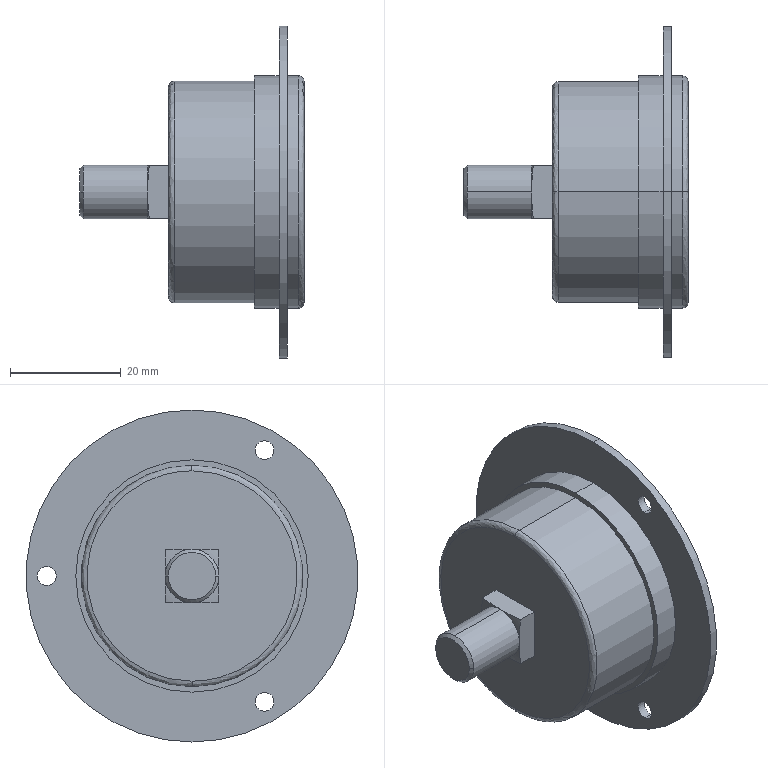Part | 1 solid | 39 faces | box 40.5 x 60 x 60 mm | volume 34153 mm3 | cylinder 18 | plane 11 | spline 4 | torus 4 | cone 2 | commonest cylinder face diameters 3.4 x6 42 x4 9.728 x2 37.8 x2 40 x2 60 x2
STEP:
#1=CARTESIAN_POINT('',(1.,0.,20.));
#2=VERTEX_POINT('',#1);
#3=CARTESIAN_POINT('',(1.,0.,-20.));
#4=VERTEX_POINT('',#3);
#5=CARTESIAN_POINT('',(1.,0.,0.));
#6=DIRECTION('',(1.,0.,0.));
#7=DIRECTION('',(0.,0.,1.));
#8=AXIS2_PLACEMENT_3D('',#5,#6,#7);
#9=CIRCLE('',#8,20.);
#10=EDGE_CURVE('',#2,#4,#9,.T.);
#11=ORIENTED_EDGE('',*,*,#10,.F.);
#12=CARTESIAN_POINT('',(0.,0.,19.));
#13=VERTEX_POINT('',#12);
#14=CARTESIAN_POINT('',(1.,0.,19.));
#15=DIRECTION('',(0.,-1.,0.));
#16=DIRECTION('',(0.,0.,1.));
#17=AXIS2_PLACEMENT_3D('',#14,#15,#16);
#18=CIRCLE('',#17,1.);
#19=EDGE_CURVE('',#2,#13,#18,.T.);
#20=ORIENTED_EDGE('',*,*,#19,.T.);
#21=CARTESIAN_POINT('',(0.,0.,-19.));
#22=VERTEX_POINT('',#21);
#23=CARTESIAN_POINT('',(0.,0.,19.));
#24=CARTESIAN_POINT('',(0.,-38.,19.));
#25=CARTESIAN_POINT('',(0.,-38.,-19.));
#26=CARTESIAN_POINT('',(0.,0.,-19.));
#27=(BOUNDED_CURVE()B_SPLINE_CURVE(3,(#23,#24,#25,#26),.UNSPECIFIED.,.F.,.F.)B_SPLINE_CURVE_WITH_KNOTS((4,4),(0.5,1.),.UNSPECIFIED.)CURVE()GEOMETRIC_REPRESENTATION_ITEM()RATIONAL_B_SPLINE_CURVE((1.,0.3333,0.3333,1.))REPRESENTATION_ITEM(''));
#28=EDGE_CURVE('',#13,#22,#27,.T.);
#29=ORIENTED_EDGE('',*,*,#28,.T.);
#30=CARTESIAN_POINT('',(1.,0.,-19.));
#31=DIRECTION('',(0.,1.,0.));
#32=DIRECTION('',(0.,0.,-1.));
#33=AXIS2_PLACEMENT_3D('',#30,#31,#32);
#34=CIRCLE('',#33,1.);
#35=EDGE_CURVE('',#4,#22,#34,.T.);
#36=ORIENTED_EDGE('',*,*,#35,.F.);
#37=EDGE_LOOP('',(#11,#20,#29,#36));
#38=FACE_OUTER_BOUND('',#37,.T.);
#39=CARTESIAN_POINT('',(1.,0.,20.));
#40=CARTESIAN_POINT('',(1.,-40.,20.));
#41=CARTESIAN_POINT('',(1.,-40.,-20.));
#42=CARTESIAN_POINT('',(1.,0.,-20.));
#43=CARTESIAN_POINT('',(0.4142,0.,20.));
#44=CARTESIAN_POINT('',(0.4142,-40.,20.));
#45=CARTESIAN_POINT('',(0.4142,-40.,-20.));
#46=CARTESIAN_POINT('',(0.4142,0.,-20.));
#47=CARTESIAN_POINT('',(0.,0.,19.586));
#48=CARTESIAN_POINT('',(0.,-39.172,19.586));
#49=CARTESIAN_POINT('',(0.,-39.172,-19.586));
#50=CARTESIAN_POINT('',(0.,0.,-19.586));
#51=CARTESIAN_POINT('',(0.,0.,19.));
#52=CARTESIAN_POINT('',(0.,-38.,19.));
#53=CARTESIAN_POINT('',(0.,-38.,-19.));
#54=CARTESIAN_POINT('',(0.,0.,-19.));
#55=(BOUNDED_SURFACE()B_SPLINE_SURFACE(3,3,((#39,#40,#41,#42),(#43,#44,#45,#46),(#47,#48,#49,#50),(#51,#52,#53,#54)),.UNSPECIFIED.,.F.,.F.,.T.)B_SPLINE_SURFACE_WITH_KNOTS((4,4),(4,4),(0.,1.),(0.,1.),.UNSPECIFIED.)GEOMETRIC_REPRESENTATION_ITEM()RATIONAL_B_SPLINE_SURFACE(((1.,0.3333,0.3333,1.),(0.8047,0.2682,0.2682,0.8047),(0.8047,0.2682,0.2682,0.8047),(1.,0.3333,0.3333,1.)))REPRESENTATION_ITEM('')SURFACE());
#56=ADVANCED_FACE('',(#38),#55,.T.);
#57=CARTESIAN_POINT('',(24.5,0.,-20.));
#58=VERTEX_POINT('',#57);
#59=CARTESIAN_POINT('',(24.5,0.,20.));
#60=VERTEX_POINT('',#59);
#61=CARTESIAN_POINT('',(24.5,0.,-20.));
#62=CARTESIAN_POINT('',(24.5,-40.,-20.));
#63=CARTESIAN_POINT('',(24.5,-40.,20.));
#64=CARTESIAN_POINT('',(24.5,0.,20.));
#65=(BOUNDED_CURVE()B_SPLINE_CURVE(3,(#61,#62,#63,#64),.UNSPECIFIED.,.F.,.F.)B_SPLINE_CURVE_WITH_KNOTS((4,4),(0.,0.5),.UNSPECIFIED.)CURVE()GEOMETRIC_REPRESENTATION_ITEM()RATIONAL_B_SPLINE_CURVE((1.,0.3333,0.3333,1.))REPRESENTATION_ITEM(''));
#66=EDGE_CURVE('',#58,#60,#65,.T.);
#67=ORIENTED_EDGE('',*,*,#66,.T.);
#68=CARTESIAN_POINT('',(23.5,0.,21.));
#69=VERTEX_POINT('',#68);
#70=CARTESIAN_POINT('',(23.5,0.,20.));
#71=DIRECTION('',(0.,-1.,0.));
#72=DIRECTION('',(0.,0.,1.));
#73=AXIS2_PLACEMENT_3D('',#70,#71,#72);
#74=CIRCLE('',#73,1.);
#75=EDGE_CURVE('',#60,#69,#74,.T.);
#76=ORIENTED_EDGE('',*,*,#75,.T.);
#77=CARTESIAN_POINT('',(23.5,0.,-21.));
#78=VERTEX_POINT('',#77);
#79=CARTESIAN_POINT('',(23.5,0.,0.));
#80=DIRECTION('',(-1.,0.,0.));
#81=DIRECTION('',(0.,0.,1.));
#82=AXIS2_PLACEMENT_3D('',#79,#80,#81);
#83=CIRCLE('',#82,21.);
#84=EDGE_CURVE('',#78,#69,#83,.T.);
#85=ORIENTED_EDGE('',*,*,#84,.F.);
#86=CARTESIAN_POINT('',(23.5,0.,-20.));
#87=DIRECTION('',(0.,1.,0.));
#88=DIRECTION('',(0.,0.,-1.));
#89=AXIS2_PLACEMENT_3D('',#86,#87,#88);
#90=CIRCLE('',#89,1.);
#91=EDGE_CURVE('',#58,#78,#90,.T.);
#92=ORIENTED_EDGE('',*,*,#91,.F.);
#93=EDGE_LOOP('',(#67,#76,#85,#92));
#94=FACE_OUTER_BOUND('',#93,.T.);
#95=CARTESIAN_POINT('',(24.5,0.,20.));
#96=CARTESIAN_POINT('',(24.5,-40.,20.));
#97=CARTESIAN_POINT('',(24.5,-40.,-20.));
#98=CARTESIAN_POINT('',(24.5,0.,-20.));
#99=CARTESIAN_POINT('',(24.5,0.,20.586));
#100=CARTESIAN_POINT('',(24.5,-41.172,20.586));
#101=CARTESIAN_POINT('',(24.5,-41.172,-20.586));
#102=CARTESIAN_POINT('',(24.5,0.,-20.586));
#103=CARTESIAN_POINT('',(24.086,0.,21.));
#104=CARTESIAN_POINT('',(24.086,-42.,21.));
#105=CARTESIAN_POINT('',(24.086,-42.,-21.));
#106=CARTESIAN_POINT('',(24.086,0.,-21.));
#107=CARTESIAN_POINT('',(23.5,0.,21.));
#108=CARTESIAN_POINT('',(23.5,-42.,21.));
#109=CARTESIAN_POINT('',(23.5,-42.,-21.));
#110=CARTESIAN_POINT('',(23.5,0.,-21.));
#111=(BOUNDED_SURFACE()B_SPLINE_SURFACE(3,3,((#95,#96,#97,#98),(#99,#100,#101,#102),(#103,#104,#105,#106),(#107,#108,#109,#110)),.UNSPECIFIED.,.F.,.F.,.F.)B_SPLINE_SURFACE_WITH_KNOTS((4,4),(4,4),(0.,1.),(0.,1.),.UNSPECIFIED.)GEOMETRIC_REPRESENTATION_ITEM()RATIONAL_B_SPLINE_SURFACE(((1.,0.3333,0.3333,1.),(0.8047,0.2682,0.2682,0.8047),(0.8047,0.2682,0.2682,0.8047),(1.,0.3333,0.3333,1.)))REPRESENTATION_ITEM('')SURFACE());
#112=ADVANCED_FACE('',(#94),#111,.T.);
#113=CARTESIAN_POINT('',(15.5,0.,20.));
#114=VERTEX_POINT('',#113);
#115=CARTESIAN_POINT('',(15.5,0.,-20.));
#116=VERTEX_POINT('',#115);
#117=CARTESIAN_POINT('',(15.5,0.,0.));
#118=DIRECTION('',(-1.,0.,0.));
#119=DIRECTION('',(0.,0.,1.));
#120=AXIS2_PLACEMENT_3D('',#117,#118,#119);
#121=CIRCLE('',#120,20.);
#122=EDGE_CURVE('',#114,#116,#121,.T.);
#123=ORIENTED_EDGE('',*,*,#122,.T.);
#124=CARTESIAN_POINT('',(23.5,0.,-20.));
#125=DIRECTION('',(-1.,0.,0.));
#126=VECTOR('',#125,1000.);
#127=LINE('',#124,#126);
#128=EDGE_CURVE('',#116,#4,#127,.T.);
#129=ORIENTED_EDGE('',*,*,#128,.T.);
#130=CARTESIAN_POINT('',(1.,0.,0.));
#131=DIRECTION('',(1.,0.,0.));
#132=DIRECTION('',(0.,0.,1.));
#133=AXIS2_PLACEMENT_3D('',#130,#131,#132);
#134=CIRCLE('',#133,20.);
#135=EDGE_CURVE('',#4,#2,#134,.T.);
#136=ORIENTED_EDGE('',*,*,#135,.T.);
#137=CARTESIAN_POINT('',(23.5,0.,20.));
#138=DIRECTION('',(-1.,0.,0.));
#139=VECTOR('',#138,1000.);
#140=LINE('',#137,#139);
#141=EDGE_CURVE('',#114,#2,#140,.T.);
#142=ORIENTED_EDGE('',*,*,#141,.F.);
#143=EDGE_LOOP('',(#123,#129,#136,#142));
#144=FACE_OUTER_BOUND('',#143,.T.);
#145=CARTESIAN_POINT('',(23.5,0.,0.));
#146=DIRECTION('',(-1.,0.,0.));
#147=DIRECTION('',(0.,0.,1.));
#148=AXIS2_PLACEMENT_3D('',#145,#146,#147);
#149=CYLINDRICAL_SURFACE('',#148,20.);
#150=ADVANCED_FACE('',(#144),#149,.T.);
#151=CARTESIAN_POINT('',(20.,0.,21.));
#152=VERTEX_POINT('',#151);
#153=CARTESIAN_POINT('',(20.,0.,-21.));
#154=VERTEX_POINT('',#153);
#155=CARTESIAN_POINT('',(20.,0.,0.));
#156=DIRECTION('',(-1.,0.,0.));
#157=DIRECTION('',(0.,0.,1.));
#158=AXIS2_PLACEMENT_3D('',#155,#156,#157);
#159=CIRCLE('',#158,21.);
#160=EDGE_CURVE('',#152,#154,#159,.T.);
#161=ORIENTED_EDGE('',*,*,#160,.T.);
#162=CARTESIAN_POINT('',(15.5,0.,-21.));
#163=VERTEX_POINT('',#162);
#164=CARTESIAN_POINT('',(23.5,0.,-21.));
#165=DIRECTION('',(-1.,0.,0.));
#166=VECTOR('',#165,1000.);
#167=LINE('',#164,#166);
#168=EDGE_CURVE('',#154,#163,#167,.T.);
#169=ORIENTED_EDGE('',*,*,#168,.T.);
#170=CARTESIAN_POINT('',(15.5,0.,21.));
#171=VERTEX_POINT('',#170);
#172=CARTESIAN_POINT('',(15.5,0.,0.));
#173=DIRECTION('',(1.,0.,0.));
#174=DIRECTION('',(0.,0.,1.));
#175=AXIS2_PLACEMENT_3D('',#172,#173,#174);
#176=CIRCLE('',#175,21.);
#177=EDGE_CURVE('',#163,#171,#176,.T.);
#178=ORIENTED_EDGE('',*,*,#177,.T.);
#179=CARTESIAN_POINT('',(23.5,0.,21.));
#180=DIRECTION('',(-1.,0.,0.));
#181=VECTOR('',#180,1000.);
#182=LINE('',#179,#181);
#183=EDGE_CURVE('',#152,#171,#182,.T.);
#184=ORIENTED_EDGE('',*,*,#183,.F.);
#185=EDGE_LOOP('',(#161,#169,#178,#184));
#186=FACE_OUTER_BOUND('',#185,.T.);
#187=CARTESIAN_POINT('',(23.5,0.,0.));
#188=DIRECTION('',(-1.,0.,0.));
#189=DIRECTION('',(0.,0.,1.));
#190=AXIS2_PLACEMENT_3D('',#187,#188,#189);
#191=CYLINDRICAL_SURFACE('',#190,21.);
#192=ADVANCED_FACE('',(#186),#191,.T.);
#193=CARTESIAN_POINT('',(20.,-13.125,-24.433));
#194=VERTEX_POINT('',#193);
#195=CARTESIAN_POINT('',(20.,-13.125,-21.033));
#196=VERTEX_POINT('',#195);
#197=CARTESIAN_POINT('',(20.,-13.125,-22.733));
#198=DIRECTION('',(-1.,0.,0.));
#199=DIRECTION('',(0.,0.,-1.));
#200=AXIS2_PLACEMENT_3D('',#197,#198,#199);
#201=CIRCLE('',#200,1.7);
#202=EDGE_CURVE('',#194,#196,#201,.T.);
#203=ORIENTED_EDGE('',*,*,#202,.T.);
#204=CARTESIAN_POINT('',(21.5,-13.125,-21.033));
#205=VERTEX_POINT('',#204);
#206=CARTESIAN_POINT('',(40.5,-13.125,-21.033));
#207=DIRECTION('',(1.,0.,0.));
#208=VECTOR('',#207,1000.);
#209=LINE('',#206,#208);
#210=EDGE_CURVE('',#196,#205,#209,.T.);
#211=ORIENTED_EDGE('',*,*,#210,.T.);
#212=CARTESIAN_POINT('',(21.5,-13.125,-24.433));
#213=VERTEX_POINT('',#212);
#214=CARTESIAN_POINT('',(21.5,-13.125,-22.733));
#215=DIRECTION('',(-1.,0.,0.));
#216=DIRECTION('',(0.,0.,-1.));
#217=AXIS2_PLACEMENT_3D('',#214,#215,#216);
#218=CIRCLE('',#217,1.7);
#219=EDGE_CURVE('',#213,#205,#218,.T.);
#220=ORIENTED_EDGE('',*,*,#219,.F.);
#221=CARTESIAN_POINT('',(40.5,-13.125,-24.433));
#222=DIRECTION('',(1.,0.,0.));
#223=VECTOR('',#222,1000.);
#224=LINE('',#221,#223);
#225=EDGE_CURVE('',#194,#213,#224,.T.);
#226=ORIENTED_EDGE('',*,*,#225,.F.);
#227=EDGE_LOOP('',(#203,#211,#220,#226));
#228=FACE_OUTER_BOUND('',#227,.T.);
#229=CARTESIAN_POINT('',(40.5,-13.125,-22.733));
#230=DIRECTION('',(1.,0.,0.));
#231=DIRECTION('',(0.,0.,-1.));
#232=AXIS2_PLACEMENT_3D('',#229,#230,#231);
#233=CYLINDRICAL_SURFACE('',#232,1.7);
#234=ADVANCED_FACE('',(#228),#233,.F.);
#235=CARTESIAN_POINT('',(20.,-13.125,21.033));
#236=VERTEX_POINT('',#235);
#237=CARTESIAN_POINT('',(20.,-13.125,24.433));
#238=VERTEX_POINT('',#237);
#239=CARTESIAN_POINT('',(20.,-13.125,22.733));
#240=DIRECTION('',(-1.,0.,0.));
#241=DIRECTION('',(0.,0.,-1.));
#242=AXIS2_PLACEMENT_3D('',#239,#240,#241);
#243=CIRCLE('',#242,1.7);
#244=EDGE_CURVE('',#236,#238,#243,.T.);
#245=ORIENTED_EDGE('',*,*,#244,.T.);
#246=CARTESIAN_POINT('',(21.5,-13.125,24.433));
#247=VERTEX_POINT('',#246);
#248=CARTESIAN_POINT('',(40.5,-13.125,24.433));
#249=DIRECTION('',(1.,0.,0.));
#250=VECTOR('',#249,1000.);
#251=LINE('',#248,#250);
#252=EDGE_CURVE('',#238,#247,#251,.T.);
#253=ORIENTED_EDGE('',*,*,#252,.T.);
#254=CARTESIAN_POINT('',(21.5,-13.125,21.033));
#255=VERTEX_POINT('',#254);
#256=CARTESIAN_POINT('',(21.5,-13.125,22.733));
#257=DIRECTION('',(-1.,0.,0.));
#258=DIRECTION('',(0.,0.,-1.));
#259=AXIS2_PLACEMENT_3D('',#256,#257,#258);
#260=CIRCLE('',#259,1.7);
#261=EDGE_CURVE('',#255,#247,#260,.T.);
#262=ORIENTED_EDGE('',*,*,#261,.F.);
#263=CARTESIAN_POINT('',(40.5,-13.125,21.033));
#264=DIRECTION('',(1.,0.,0.));
#265=VECTOR('',#264,1000.);
#266=LINE('',#263,#265);
#267=EDGE_CURVE('',#236,#255,#266,.T.);
#268=ORIENTED_EDGE('',*,*,#267,.F.);
#269=EDGE_LOOP('',(#245,#253,#262,#268));
#270=FACE_OUTER_BOUND('',#269,.T.);
#271=CARTESIAN_POINT('',(40.5,-13.125,22.733));
#272=DIRECTION('',(1.,0.,0.));
#273=DIRECTION('',(0.,0.,-1.));
#274=AXIS2_PLACEMENT_3D('',#271,#272,#273);
#275=CYLINDRICAL_SURFACE('',#274,1.7);
#276=ADVANCED_FACE('',(#270),#275,.F.);
#277=CARTESIAN_POINT('',(20.,26.25,-1.7));
#278=VERTEX_POINT('',#277);
#279=CARTESIAN_POINT('',(20.,26.25,1.7));
#280=VERTEX_POINT('',#279);
#281=CARTESIAN_POINT('',(20.,26.25,0.));
#282=DIRECTION('',(-1.,0.,0.));
#283=DIRECTION('',(0.,0.,-1.));
#284=AXIS2_PLACEMENT_3D('',#281,#282,#283);
#285=CIRCLE('',#284,1.7);
#286=EDGE_CURVE('',#278,#280,#285,.T.);
#287=ORIENTED_EDGE('',*,*,#286,.T.);
#288=CARTESIAN_POINT('',(21.5,26.25,1.7));
#289=VERTEX_POINT('',#288);
#290=CARTESIAN_POINT('',(40.5,26.25,1.7));
#291=DIRECTION('',(1.,0.,0.));
#292=VECTOR('',#291,1000.);
#293=LINE('',#290,#292);
#294=EDGE_CURVE('',#280,#289,#293,.T.);
#295=ORIENTED_EDGE('',*,*,#294,.T.);
#296=CARTESIAN_POINT('',(21.5,26.25,-1.7));
#297=VERTEX_POINT('',#296);
#298=CARTESIAN_POINT('',(21.5,26.25,0.));
#299=DIRECTION('',(-1.,0.,0.));
#300=DIRECTION('',(0.,0.,-1.));
#301=AXIS2_PLACEMENT_3D('',#298,#299,#300);
#302=CIRCLE('',#301,1.7);
#303=EDGE_CURVE('',#297,#289,#302,.T.);
#304=ORIENTED_EDGE('',*,*,#303,.F.);
#305=CARTESIAN_POINT('',(40.5,26.25,-1.7));
#306=DIRECTION('',(1.,0.,0.));
#307=VECTOR('',#306,1000.);
#308=LINE('',#305,#307);
#309=EDGE_CURVE('',#278,#297,#308,.T.);
#310=ORIENTED_EDGE('',*,*,#309,.F.);
#311=EDGE_LOOP('',(#287,#295,#304,#310));
#312=FACE_OUTER_BOUND('',#311,.T.);
#313=CARTESIAN_POINT('',(40.5,26.25,0.));
#314=DIRECTION('',(1.,0.,0.));
#315=DIRECTION('',(0.,0.,-1.));
#316=AXIS2_PLACEMENT_3D('',#313,#314,#315);
#317=CYLINDRICAL_SURFACE('',#316,1.7);
#318=ADVANCED_FACE('',(#312),#317,.F.);
#319=CARTESIAN_POINT('',(21.5,0.,30.));
#320=VERTEX_POINT('',#319);
#321=CARTESIAN_POINT('',(21.5,0.,-30.));
#322=VERTEX_POINT('',#321);
#323=CARTESIAN_POINT('',(21.5,0.,0.));
#324=DIRECTION('',(-1.,0.,0.));
#325=DIRECTION('',(0.,0.,1.));
#326=AXIS2_PLACEMENT_3D('',#323,#324,#325);
#327=CIRCLE('',#326,30.);
#328=EDGE_CURVE('',#320,#322,#327,.T.);
#329=ORIENTED_EDGE('',*,*,#328,.T.);
#330=CARTESIAN_POINT('',(20.,0.,-30.));
#331=VERTEX_POINT('',#330);
#332=CARTESIAN_POINT('',(23.5,0.,-30.));
#333=DIRECTION('',(-1.,0.,0.));
#334=VECTOR('',#333,1000.);
#335=LINE('',#332,#334);
#336=EDGE_CURVE('',#322,#331,#335,.T.);
#337=ORIENTED_EDGE('',*,*,#336,.T.);
#338=CARTESIAN_POINT('',(20.,0.,30.));
#339=VERTEX_POINT('',#338);
#340=CARTESIAN_POINT('',(20.,0.,0.));
#341=DIRECTION('',(1.,0.,0.));
#342=DIRECTION('',(0.,0.,1.));
#343=AXIS2_PLACEMENT_3D('',#340,#341,#342);
#344=CIRCLE('',#343,30.);
#345=EDGE_CURVE('',#331,#339,#344,.T.);
#346=ORIENTED_EDGE('',*,*,#345,.T.);
#347=CARTESIAN_POINT('',(23.5,0.,30.));
#348=DIRECTION('',(-1.,0.,0.));
#349=VECTOR('',#348,1000.);
#350=LINE('',#347,#349);
#351=EDGE_CURVE('',#320,#339,#350,.T.);
#352=ORIENTED_EDGE('',*,*,#351,.F.);
#353=EDGE_LOOP('',(#329,#337,#346,#352));
#354=FACE_OUTER_BOUND('',#353,.T.);
#355=CARTESIAN_POINT('',(23.5,0.,0.));
#356=DIRECTION('',(-1.,0.,0.));
#357=DIRECTION('',(0.,0.,1.));
#358=AXIS2_PLACEMENT_3D('',#355,#356,#357);
#359=CYLINDRICAL_SURFACE('',#358,30.);
#360=ADVANCED_FACE('',(#354),#359,.T.);
#361=CARTESIAN_POINT('',(-3.753,0.,-4.864));
#362=VERTEX_POINT('',#361);
#363=CARTESIAN_POINT('',(-3.753,4.864,0.));
#364=VERTEX_POINT('',#363);
#365=CARTESIAN_POINT('',(-3.753,0.,0.));
#366=DIRECTION('',(1.,0.,0.));
#367=DIRECTION('',(0.,1.,0.));
#368=AXIS2_PLACEMENT_3D('',#365,#366,#367);
#369=CIRCLE('',#368,4.864);
#370=EDGE_CURVE('',#362,#364,#369,.T.);
#371=ORIENTED_EDGE('',*,*,#370,.F.);
#372=CARTESIAN_POINT('',(-15.419,0.,-4.864));
#373=VERTEX_POINT('',#372);
#374=CARTESIAN_POINT('',(23.5,0.,-4.864));
#375=DIRECTION('',(-1.,0.,0.));
#376=VECTOR('',#375,1000.);
#377=LINE('',#374,#376);
#378=EDGE_CURVE('',#362,#373,#377,.T.);
#379=ORIENTED_EDGE('',*,*,#378,.T.);
#380=CARTESIAN_POINT('',(-15.419,4.864,0.));
#381=VERTEX_POINT('',#380);
#382=CARTESIAN_POINT('',(-15.419,0.,0.));
#383=DIRECTION('',(1.,0.,0.));
#384=DIRECTION('',(0.,0.,1.));
#385=AXIS2_PLACEMENT_3D('',#382,#383,#384);
#386=CIRCLE('',#385,4.864);
#387=EDGE_CURVE('',#373,#381,#386,.T.);
#388=ORIENTED_EDGE('',*,*,#387,.T.);
#389=CARTESIAN_POINT('',(-15.419,0.,4.864));
#390=VERTEX_POINT('',#389);
#391=CARTESIAN_POINT('',(-15.419,0.,0.));
#392=DIRECTION('',(1.,0.,0.));
#393=DIRECTION('',(0.,0.,1.));
#394=AXIS2_PLACEMENT_3D('',#391,#392,#393);
#395=CIRCLE('',#394,4.864);
#396=EDGE_CURVE('',#381,#390,#395,.T.);
#397=ORIENTED_EDGE('',*,*,#396,.T.);
#398=CARTESIAN_POINT('',(-3.753,0.,4.864));
#399=VERTEX_POINT('',#398);
#400=CARTESIAN_POINT('',(23.5,0.,4.864));
#401=DIRECTION('',(-1.,0.,0.));
#402=VECTOR('',#401,1000.);
#403=LINE('',#400,#402);
#404=EDGE_CURVE('',#399,#390,#403,.T.);
#405=ORIENTED_EDGE('',*,*,#404,.F.);
#406=CARTESIAN_POINT('',(-3.753,0.,0.));
#407=DIRECTION('',(1.,0.,0.));
#408=DIRECTION('',(0.,1.,0.));
#409=AXIS2_PLACEMENT_3D('',#406,#407,#408);
#410=CIRCLE('',#409,4.864);
#411=EDGE_CURVE('',#364,#399,#410,.T.);
#412=ORIENTED_EDGE('',*,*,#411,.F.);
#413=EDGE_LOOP('',(#371,#379,#388,#397,#405,#412));
#414=FACE_OUTER_BOUND('',#413,.T.);
#415=CARTESIAN_POINT('',(23.5,0.,0.));
#416=DIRECTION('',(-1.,0.,0.));
#417=DIRECTION('',(0.,0.,1.));
#418=AXIS2_PLACEMENT_3D('',#415,#416,#417);
#419=CYLINDRICAL_SURFACE('',#418,4.864);
#420=ADVANCED_FACE('',(#414),#419,.T.);
#421=CARTESIAN_POINT('',(-16.,4.283,0.));
#422=VERTEX_POINT('',#421);
#423=CARTESIAN_POINT('',(-16.,-4.283,0.));
#424=VERTEX_POINT('',#423);
#425=CARTESIAN_POINT('',(-16.,0.,0.));
#426=DIRECTION('',(1.,0.,0.));
#427=DIRECTION('',(0.,1.,0.));
#428=AXIS2_PLACEMENT_3D('',#425,#426,#427);
#429=CIRCLE('',#428,4.283);
#430=EDGE_CURVE('',#422,#424,#429,.T.);
#431=ORIENTED_EDGE('',*,*,#430,.T.);
#432=CARTESIAN_POINT('',(-15.419,-4.864,0.));
#433=VERTEX_POINT('',#432);
#434=CARTESIAN_POINT('',(-15.419,-4.864,0.));
#435=DIRECTION('',(0.7071,-0.7071,0.));
#436=VECTOR('',#435,1000.);
#437=LINE('',#434,#436);
#438=EDGE_CURVE('',#424,#433,#437,.T.);
#439=ORIENTED_EDGE('',*,*,#438,.T.);
#440=CARTESIAN_POINT('',(-15.419,0.,0.));
#441=DIRECTION('',(1.,0.,0.));
#442=DIRECTION('',(0.,0.,1.));
#443=AXIS2_PLACEMENT_3D('',#440,#441,#442);
#444=CIRCLE('',#443,4.864);
#445=EDGE_CURVE('',#390,#433,#444,.T.);
#446=ORIENTED_EDGE('',*,*,#445,.F.);
#447=ORIENTED_EDGE('',*,*,#396,.F.);
#448=CARTESIAN_POINT('',(-15.419,4.864,0.));
#449=DIRECTION('',(0.7071,0.7071,0.));
#450=VECTOR('',#449,1000.);
#451=LINE('',#448,#450);
#452=EDGE_CURVE('',#422,#381,#451,.T.);
#453=ORIENTED_EDGE('',*,*,#452,.F.);
#454=EDGE_LOOP('',(#431,#439,#446,#447,#453));
#455=FACE_OUTER_BOUND('',#454,.T.);
#456=CARTESIAN_POINT('',(-15.419,0.,0.));
#457=DIRECTION('',(1.,0.,0.));
#458=DIRECTION('',(0.,1.,0.));
#459=AXIS2_PLACEMENT_3D('',#456,#457,#458);
#460=CONICAL_SURFACE('',#459,4.864,0.7854);
#461=ADVANCED_FACE('',(#455),#460,.T.);
#462=CARTESIAN_POINT('',(23.5,0.,0.));
#463=DIRECTION('',(-1.,0.,0.));
#464=DIRECTION('',(0.,0.,1.));
#465=AXIS2_PLACEMENT_3D('',#462,#463,#464);
#466=CIRCLE('',#465,21.);
#467=EDGE_CURVE('',#69,#78,#466,.T.);
#468=ORIENTED_EDGE('',*,*,#467,.T.);
#469=CARTESIAN_POINT('',(21.5,0.,-21.));
#470=VERTEX_POINT('',#469);
#471=CARTESIAN_POINT('',(23.5,0.,-21.));
#472=DIRECTION('',(-1.,0.,0.));
#473=VECTOR('',#472,1000.);
#474=LINE('',#471,#473);
#475=EDGE_CURVE('',#78,#470,#474,.T.);
#476=ORIENTED_EDGE('',*,*,#475,.T.);
#477=CARTESIAN_POINT('',(21.5,0.,21.));
#478=VERTEX_POINT('',#477);
#479=CARTESIAN_POINT('',(21.5,0.,0.));
#480=DIRECTION('',(1.,0.,0.));
#481=DIRECTION('',(0.,0.,1.));
#482=AXIS2_PLACEMENT_3D('',#479,#480,#481);
#483=CIRCLE('',#482,21.);
#484=EDGE_CURVE('',#470,#478,#483,.T.);
#485=ORIENTED_EDGE('',*,*,#484,.T.);
#486=CARTESIAN_POINT('',(23.5,0.,21.));
#487=DIRECTION('',(-1.,0.,0.));
#488=VECTOR('',#487,1000.);
#489=LINE('',#486,#488);
#490=EDGE_CURVE('',#69,#478,#489,.T.);
#491=ORIENTED_EDGE('',*,*,#490,.F.);
#492=EDGE_LOOP('',(#468,#476,#485,#491));
#493=FACE_OUTER_BOUND('',#492,.T.);
#494=CARTESIAN_POINT('',(23.5,0.,0.));
#495=DIRECTION('',(-1.,0.,0.));
#496=DIRECTION('',(0.,0.,1.));
#497=AXIS2_PLACEMENT_3D('',#494,#495,#496);
#498=CYLINDRICAL_SURFACE('',#497,21.);
#499=ADVANCED_FACE('',(#493),#498,.T.);
#500=CARTESIAN_POINT('',(24.5,0.,18.9));
#501=VERTEX_POINT('',#500);
#502=CARTESIAN_POINT('',(24.5,0.,-18.9));
#503=VERTEX_POINT('',#502);
#504=CARTESIAN_POINT('',(24.5,0.,0.));
#505=DIRECTION('',(1.,0.,0.));
#506=DIRECTION('',(0.,0.,1.));
#507=AXIS2_PLACEMENT_3D('',#504,#505,#506);
#508=CIRCLE('',#507,18.9);
#509=EDGE_CURVE('',#501,#503,#508,.T.);
#510=ORIENTED_EDGE('',*,*,#509,.T.);
#511=CARTESIAN_POINT('',(23.5,0.,-18.9));
#512=VERTEX_POINT('',#511);
#513=CARTESIAN_POINT('',(23.5,0.,-18.9));
#514=DIRECTION('',(-1.,0.,0.));
#515=VECTOR('',#514,1000.);
#516=LINE('',#513,#515);
#517=EDGE_CURVE('',#503,#512,#516,.T.);
#518=ORIENTED_EDGE('',*,*,#517,.T.);
#519=CARTESIAN_POINT('',(23.5,0.,18.9));
#520=VERTEX_POINT('',#519);
#521=CARTESIAN_POINT('',(23.5,0.,0.));
#522=DIRECTION('',(1.,0.,0.));
#523=DIRECTION('',(0.,0.,1.));
#524=AXIS2_PLACEMENT_3D('',#521,#522,#523);
#525=CIRCLE('',#524,18.9);
#526=EDGE_CURVE('',#520,#512,#525,.T.);
#527=ORIENTED_EDGE('',*,*,#526,.F.);
#528=CARTESIAN_POINT('',(23.5,0.,18.9));
#529=DIRECTION('',(-1.,0.,0.));
#530=VECTOR('',#529,1000.);
#531=LINE('',#528,#530);
#532=EDGE_CURVE('',#501,#520,#531,.T.);
#533=ORIENTED_EDGE('',*,*,#532,.F.);
#534=EDGE_LOOP('',(#510,#518,#527,#533));
#535=FACE_OUTER_BOUND('',#534,.T.);
#536=CARTESIAN_POINT('',(23.5,0.,0.));
#537=DIRECTION('',(-1.,0.,0.));
#538=DIRECTION('',(0.,0.,1.));
#539=AXIS2_PLACEMENT_3D('',#536,#537,#538);
#540=CYLINDRICAL_SURFACE('',#539,18.9);
#541=ADVANCED_FACE('',(#535),#540,.F.);
#542=ORIENTED_EDGE('',*,*,#128,.F.);
#543=CARTESIAN_POINT('',(15.5,0.,0.));
#544=DIRECTION('',(-1.,0.,0.));
#545=DIRECTION('',(0.,0.,1.));
#546=AXIS2_PLACEMENT_3D('',#543,#544,#545);
#547=CIRCLE('',#546,20.);
#548=EDGE_CURVE('',#116,#114,#547,.T.);
#549=ORIENTED_EDGE('',*,*,#548,.T.);
#550=ORIENTED_EDGE('',*,*,#141,.T.);
#551=ORIENTED_EDGE('',*,*,#10,.T.);
#552=EDGE_LOOP('',(#542,#549,#550,#551));
#553=FACE_OUTER_BOUND('',#552,.T.);
#554=CARTESIAN_POINT('',(23.5,0.,0.));
#555=DIRECTION('',(-1.,0.,0.));
#556=DIRECTION('',(0.,0.,1.));
#557=AXIS2_PLACEMENT_3D('',#554,#555,#556);
#558=CYLINDRICAL_SURFACE('',#557,20.);
#559=ADVANCED_FACE('',(#553),#558,.T.);
#560=ORIENTED_EDGE('',*,*,#19,.F.);
#561=ORIENTED_EDGE('',*,*,#135,.F.);
#562=ORIENTED_EDGE('',*,*,#35,.T.);
#563=CARTESIAN_POINT('',(0.,0.,-19.));
#564=CARTESIAN_POINT('',(0.,38.,-19.));
#565=CARTESIAN_POINT('',(0.,38.,19.));
#566=CARTESIAN_POINT('',(0.,0.,19.));
#567=(BOUNDED_CURVE()B_SPLINE_CURVE(3,(#563,#564,#565,#566),.UNSPECIFIED.,.F.,.F.)B_SPLINE_CURVE_WITH_KNOTS((4,4),(0.,0.5),.UNSPECIFIED.)CURVE()GEOMETRIC_REPRESENTATION_ITEM()RATIONAL_B_SPLINE_CURVE((1.,0.3333,0.3333,1.))REPRESENTATION_ITEM(''));
#568=EDGE_CURVE('',#22,#13,#567,.T.);
#569=ORIENTED_EDGE('',*,*,#568,.T.);
#570=EDGE_LOOP('',(#560,#561,#562,#569));
#571=FACE_OUTER_BOUND('',#570,.T.);
#572=CARTESIAN_POINT('',(1.,0.,-20.));
#573=CARTESIAN_POINT('',(1.,40.,-20.));
#574=CARTESIAN_POINT('',(1.,40.,20.));
#575=CARTESIAN_POINT('',(1.,0.,20.));
#576=CARTESIAN_POINT('',(0.4142,0.,-20.));
#577=CARTESIAN_POINT('',(0.4142,40.,-20.));
#578=CARTESIAN_POINT('',(0.4142,40.,20.));
#579=CARTESIAN_POINT('',(0.4142,0.,20.));
#580=CARTESIAN_POINT('',(0.,0.,-19.586));
#581=CARTESIAN_POINT('',(0.,39.172,-19.586));
#582=CARTESIAN_POINT('',(0.,39.172,19.586));
#583=CARTESIAN_POINT('',(0.,0.,19.586));
#584=CARTESIAN_POINT('',(0.,0.,-19.));
#585=CARTESIAN_POINT('',(0.,38.,-19.));
#586=CARTESIAN_POINT('',(0.,38.,19.));
#587=CARTESIAN_POINT('',(0.,0.,19.));
#588=(BOUNDED_SURFACE()B_SPLINE_SURFACE(3,3,((#572,#573,#574,#575),(#576,#577,#578,#579),(#580,#581,#582,#583),(#584,#585,#586,#587)),.UNSPECIFIED.,.F.,.F.,.F.)B_SPLINE_SURFACE_WITH_KNOTS((4,4),(4,4),(0.,1.),(0.,1.),.UNSPECIFIED.)GEOMETRIC_REPRESENTATION_ITEM()RATIONAL_B_SPLINE_SURFACE(((1.,0.3333,0.3333,1.),(0.8047,0.2682,0.2682,0.8047),(0.8047,0.2682,0.2682,0.8047),(1.,0.3333,0.3333,1.)))REPRESENTATION_ITEM('')SURFACE());
#589=ADVANCED_FACE('',(#571),#588,.T.);
#590=ORIENTED_EDGE('',*,*,#122,.F.);
#591=ORIENTED_EDGE('',*,*,#548,.F.);
#592=EDGE_LOOP('',(#590,#591));
#593=FACE_BOUND('',#592,.T.);
#594=CARTESIAN_POINT('',(15.5,0.,0.));
#595=DIRECTION('',(1.,0.,0.));
#596=DIRECTION('',(0.,0.,1.));
#597=AXIS2_PLACEMENT_3D('',#594,#595,#596);
#598=CIRCLE('',#597,21.);
#599=EDGE_CURVE('',#171,#163,#598,.T.);
#600=ORIENTED_EDGE('',*,*,#599,.F.);
#601=ORIENTED_EDGE('',*,*,#177,.F.);
#602=EDGE_LOOP('',(#600,#601));
#603=FACE_OUTER_BOUND('',#602,.T.);
#604=CARTESIAN_POINT('',(15.5,20.,0.));
#605=DIRECTION('',(1.,0.,0.));
#606=DIRECTION('',(0.,0.,-1.));
#607=AXIS2_PLACEMENT_3D('',#604,#605,#606);
#608=PLANE('',#607);
#609=ADVANCED_FACE('',(#593,#603),#608,.F.);
#610=CARTESIAN_POINT('',(0.,-4.864,4.864));
#611=VERTEX_POINT('',#610);
#612=CARTESIAN_POINT('',(0.,4.864,4.864));
#613=VERTEX_POINT('',#612);
#614=CARTESIAN_POINT('',(0.,4.864,4.864));
#615=DIRECTION('',(0.,1.,0.));
#616=VECTOR('',#615,1000.);
#617=LINE('',#614,#616);
#618=EDGE_CURVE('',#611,#613,#617,.T.);
#619=ORIENTED_EDGE('',*,*,#618,.F.);
#620=CARTESIAN_POINT('',(0.,-4.864,-4.864));
#621=VERTEX_POINT('',#620);
#622=CARTESIAN_POINT('',(0.,-4.864,0.));
#623=DIRECTION('',(0.,0.,1.));
#624=VECTOR('',#623,1000.);
#625=LINE('',#622,#624);
#626=EDGE_CURVE('',#621,#611,#625,.T.);
#627=ORIENTED_EDGE('',*,*,#626,.F.);
#628=CARTESIAN_POINT('',(0.,4.864,-4.864));
#629=VERTEX_POINT('',#628);
#630=CARTESIAN_POINT('',(0.,4.864,-4.864));
#631=DIRECTION('',(0.,-1.,0.));
#632=VECTOR('',#631,1000.);
#633=LINE('',#630,#632);
#634=EDGE_CURVE('',#629,#621,#633,.T.);
#635=ORIENTED_EDGE('',*,*,#634,.F.);
#636=CARTESIAN_POINT('',(0.,4.864,0.));
#637=DIRECTION('',(0.,0.,-1.));
#638=VECTOR('',#637,1000.);
#639=LINE('',#636,#638);
#640=EDGE_CURVE('',#613,#629,#639,.T.);
#641=ORIENTED_EDGE('',*,*,#640,.F.);
#642=EDGE_LOOP('',(#619,#627,#635,#641));
#643=FACE_BOUND('',#642,.T.);
#644=ORIENTED_EDGE('',*,*,#568,.F.);
#645=ORIENTED_EDGE('',*,*,#28,.F.);
#646=EDGE_LOOP('',(#644,#645));
#647=FACE_OUTER_BOUND('',#646,.T.);
#648=CARTESIAN_POINT('',(0.,4.864,0.));
#649=DIRECTION('',(1.,0.,0.));
#650=DIRECTION('',(0.,0.,-1.));
#651=AXIS2_PLACEMENT_3D('',#648,#649,#650);
#652=PLANE('',#651);
#653=ADVANCED_FACE('',(#643,#647),#652,.F.);
#654=ORIENTED_EDGE('',*,*,#168,.F.);
#655=CARTESIAN_POINT('',(20.,0.,0.));
#656=DIRECTION('',(-1.,0.,0.));
#657=DIRECTION('',(0.,0.,1.));
#658=AXIS2_PLACEMENT_3D('',#655,#656,#657);
#659=CIRCLE('',#658,21.);
#660=EDGE_CURVE('',#154,#152,#659,.T.);
#661=ORIENTED_EDGE('',*,*,#660,.T.);
#662=ORIENTED_EDGE('',*,*,#183,.T.);
#663=ORIENTED_EDGE('',*,*,#599,.T.);
#664=EDGE_LOOP('',(#654,#661,#662,#663));
#665=FACE_OUTER_BOUND('',#664,.T.);
#666=CARTESIAN_POINT('',(23.5,0.,0.));
#667=DIRECTION('',(-1.,0.,0.));
#668=DIRECTION('',(0.,0.,1.));
#669=AXIS2_PLACEMENT_3D('',#666,#667,#668);
#670=CYLINDRICAL_SURFACE('',#669,21.);
#671=ADVANCED_FACE('',(#665),#670,.T.);
#672=CARTESIAN_POINT('',(-3.462,4.864,-4.864));
#673=VERTEX_POINT('',#672);
#674=CARTESIAN_POINT('',(-8.,4.864,-4.864));
#675=DIRECTION('',(-1.,0.,0.));
#676=VECTOR('',#675,1000.);
#677=LINE('',#674,#676);
#678=EDGE_CURVE('',#629,#673,#677,.T.);
#679=ORIENTED_EDGE('',*,*,#678,.T.);
#680=CARTESIAN_POINT('',(-3.462,4.864,-4.864));
#681=CARTESIAN_POINT('',(-3.688,4.864,-3.25));
#682=CARTESIAN_POINT('',(-3.753,4.864,-1.627));
#683=CARTESIAN_POINT('',(-3.753,4.864,0.));
#684=B_SPLINE_CURVE_WITH_KNOTS('',3,(#680,#681,#682,#683),.UNSPECIFIED.,.F.,.F.,(4,4),(0.,0.004873),.UNSPECIFIED.);
#685=EDGE_CURVE('',#673,#364,#684,.T.);
#686=ORIENTED_EDGE('',*,*,#685,.T.);
#687=CARTESIAN_POINT('',(-3.462,4.864,4.864));
#688=VERTEX_POINT('',#687);
#689=CARTESIAN_POINT('',(-3.753,4.864,0.));
#690=CARTESIAN_POINT('',(-3.753,4.864,1.627));
#691=CARTESIAN_POINT('',(-3.688,4.864,3.25));
#692=CARTESIAN_POINT('',(-3.462,4.864,4.864));
#693=B_SPLINE_CURVE_WITH_KNOTS('',3,(#689,#690,#691,#692),.UNSPECIFIED.,.F.,.F.,(4,4),(0.,0.004873),.UNSPECIFIED.);
#694=EDGE_CURVE('',#364,#688,#693,.T.);
#695=ORIENTED_EDGE('',*,*,#694,.T.);
#696=CARTESIAN_POINT('',(-8.,4.864,4.864));
#697=DIRECTION('',(1.,0.,0.));
#698=VECTOR('',#697,1000.);
#699=LINE('',#696,#698);
#700=EDGE_CURVE('',#688,#613,#699,.T.);
#701=ORIENTED_EDGE('',*,*,#700,.T.);
#702=ORIENTED_EDGE('',*,*,#640,.T.);
#703=EDGE_LOOP('',(#679,#686,#695,#701,#702));
#704=FACE_OUTER_BOUND('',#703,.T.);
#705=CARTESIAN_POINT('',(-8.,4.864,-4.864));
#706=DIRECTION('',(0.,1.,0.));
#707=DIRECTION('',(0.,0.,1.));
#708=AXIS2_PLACEMENT_3D('',#705,#706,#707);
#709=PLANE('',#708);
#710=ADVANCED_FACE('',(#704),#709,.T.);
#711=ORIENTED_EDGE('',*,*,#700,.F.);
#712=CARTESIAN_POINT('',(-3.462,4.864,4.864));
#713=CARTESIAN_POINT('',(-3.688,3.25,4.864));
#714=CARTESIAN_POINT('',(-3.753,1.627,4.864));
#715=CARTESIAN_POINT('',(-3.753,0.,4.864));
#716=B_SPLINE_CURVE_WITH_KNOTS('',3,(#712,#713,#714,#715),.UNSPECIFIED.,.F.,.F.,(4,4),(0.,0.004873),.UNSPECIFIED.);
#717=EDGE_CURVE('',#688,#399,#716,.T.);
#718=ORIENTED_EDGE('',*,*,#717,.T.);
#719=CARTESIAN_POINT('',(-3.462,-4.864,4.864));
#720=VERTEX_POINT('',#719);
#721=CARTESIAN_POINT('',(-3.753,0.,4.864));
#722=CARTESIAN_POINT('',(-3.753,-1.627,4.864));
#723=CARTESIAN_POINT('',(-3.688,-3.25,4.864));
#724=CARTESIAN_POINT('',(-3.462,-4.864,4.864));
#725=B_SPLINE_CURVE_WITH_KNOTS('',3,(#721,#722,#723,#724),.UNSPECIFIED.,.F.,.F.,(4,4),(0.,0.004873),.UNSPECIFIED.);
#726=EDGE_CURVE('',#399,#720,#725,.T.);
#727=ORIENTED_EDGE('',*,*,#726,.T.);
#728=CARTESIAN_POINT('',(-8.,-4.864,4.864));
#729=DIRECTION('',(1.,0.,0.));
#730=VECTOR('',#729,1000.);
#731=LINE('',#728,#730);
#732=EDGE_CURVE('',#720,#611,#731,.T.);
#733=ORIENTED_EDGE('',*,*,#732,.T.);
#734=ORIENTED_EDGE('',*,*,#618,.T.);
#735=EDGE_LOOP('',(#711,#718,#727,#733,#734));
#736=FACE_OUTER_BOUND('',#735,.T.);
#737=CARTESIAN_POINT('',(-8.,4.864,4.864));
#738=DIRECTION('',(0.,0.,1.));
#739=DIRECTION('',(1.,0.,0.));
#740=AXIS2_PLACEMENT_3D('',#737,#738,#739);
#741=PLANE('',#740);
#742=ADVANCED_FACE('',(#736),#741,.T.);
#743=ORIENTED_EDGE('',*,*,#732,.F.);
#744=CARTESIAN_POINT('',(-3.753,-4.864,0.));
#745=VERTEX_POINT('',#744);
#746=CARTESIAN_POINT('',(-3.462,-4.864,4.864));
#747=CARTESIAN_POINT('',(-3.688,-4.864,3.25));
#748=CARTESIAN_POINT('',(-3.753,-4.864,1.627));
#749=CARTESIAN_POINT('',(-3.753,-4.864,0.));
#750=B_SPLINE_CURVE_WITH_KNOTS('',3,(#746,#747,#748,#749),.UNSPECIFIED.,.F.,.F.,(4,4),(0.,0.004873),.UNSPECIFIED.);
#751=EDGE_CURVE('',#720,#745,#750,.T.);
#752=ORIENTED_EDGE('',*,*,#751,.T.);
#753=CARTESIAN_POINT('',(-3.462,-4.864,-4.864));
#754=VERTEX_POINT('',#753);
#755=CARTESIAN_POINT('',(-3.753,-4.864,0.));
#756=CARTESIAN_POINT('',(-3.753,-4.864,-1.627));
#757=CARTESIAN_POINT('',(-3.688,-4.864,-3.25));
#758=CARTESIAN_POINT('',(-3.462,-4.864,-4.864));
#759=B_SPLINE_CURVE_WITH_KNOTS('',3,(#755,#756,#757,#758),.UNSPECIFIED.,.F.,.F.,(4,4),(0.,0.004873),.UNSPECIFIED.);
#760=EDGE_CURVE('',#745,#754,#759,.T.);
#761=ORIENTED_EDGE('',*,*,#760,.T.);
#762=CARTESIAN_POINT('',(-8.,-4.864,-4.864));
#763=DIRECTION('',(1.,0.,0.));
#764=VECTOR('',#763,1000.);
#765=LINE('',#762,#764);
#766=EDGE_CURVE('',#754,#621,#765,.T.);
#767=ORIENTED_EDGE('',*,*,#766,.T.);
#768=ORIENTED_EDGE('',*,*,#626,.T.);
#769=EDGE_LOOP('',(#743,#752,#761,#767,#768));
#770=FACE_OUTER_BOUND('',#769,.T.);
#771=CARTESIAN_POINT('',(-8.,-4.864,4.864));
#772=DIRECTION('',(0.,-1.,0.));
#773=DIRECTION('',(0.,0.,-1.));
#774=AXIS2_PLACEMENT_3D('',#771,#772,#773);
#775=PLANE('',#774);
#776=ADVANCED_FACE('',(#770),#775,.T.);
#777=ORIENTED_EDGE('',*,*,#766,.F.);
#778=CARTESIAN_POINT('',(-3.462,-4.864,-4.864));
#779=CARTESIAN_POINT('',(-3.688,-3.25,-4.864));
#780=CARTESIAN_POINT('',(-3.753,-1.627,-4.864));
#781=CARTESIAN_POINT('',(-3.753,0.,-4.864));
#782=B_SPLINE_CURVE_WITH_KNOTS('',3,(#778,#779,#780,#781),.UNSPECIFIED.,.F.,.F.,(4,4),(0.,0.004873),.UNSPECIFIED.);
#783=EDGE_CURVE('',#754,#362,#782,.T.);
#784=ORIENTED_EDGE('',*,*,#783,.T.);
#785=CARTESIAN_POINT('',(-3.753,0.,-4.864));
#786=CARTESIAN_POINT('',(-3.753,1.627,-4.864));
#787=CARTESIAN_POINT('',(-3.688,3.25,-4.864));
#788=CARTESIAN_POINT('',(-3.462,4.864,-4.864));
#789=B_SPLINE_CURVE_WITH_KNOTS('',3,(#785,#786,#787,#788),.UNSPECIFIED.,.F.,.F.,(4,4),(0.,0.004873),.UNSPECIFIED.);
#790=EDGE_CURVE('',#362,#673,#789,.T.);
#791=ORIENTED_EDGE('',*,*,#790,.T.);
#792=ORIENTED_EDGE('',*,*,#678,.F.);
#793=ORIENTED_EDGE('',*,*,#634,.T.);
#794=EDGE_LOOP('',(#777,#784,#791,#792,#793));
#795=FACE_OUTER_BOUND('',#794,.T.);
#796=CARTESIAN_POINT('',(-8.,-4.864,-4.864));
#797=DIRECTION('',(0.,0.,-1.));
#798=DIRECTION('',(-1.,0.,0.));
#799=AXIS2_PLACEMENT_3D('',#796,#797,#798);
#800=PLANE('',#799);
#801=ADVANCED_FACE('',(#795),#800,.T.);
#802=ORIENTED_EDGE('',*,*,#202,.F.);
#803=CARTESIAN_POINT('',(20.,-13.125,-22.733));
#804=DIRECTION('',(-1.,0.,0.));
#805=DIRECTION('',(0.,0.,-1.));
#806=AXIS2_PLACEMENT_3D('',#803,#804,#805);
#807=CIRCLE('',#806,1.7);
#808=EDGE_CURVE('',#196,#194,#807,.T.);
#809=ORIENTED_EDGE('',*,*,#808,.F.);
#810=EDGE_LOOP('',(#802,#809));
#811=FACE_BOUND('',#810,.T.);
#812=ORIENTED_EDGE('',*,*,#160,.F.);
#813=ORIENTED_EDGE('',*,*,#660,.F.);
#814=EDGE_LOOP('',(#812,#813));
#815=FACE_BOUND('',#814,.T.);
#816=ORIENTED_EDGE('',*,*,#244,.F.);
#817=CARTESIAN_POINT('',(20.,-13.125,22.733));
#818=DIRECTION('',(-1.,0.,0.));
#819=DIRECTION('',(0.,0.,-1.));
#820=AXIS2_PLACEMENT_3D('',#817,#818,#819);
#821=CIRCLE('',#820,1.7);
#822=EDGE_CURVE('',#238,#236,#821,.T.);
#823=ORIENTED_EDGE('',*,*,#822,.F.);
#824=EDGE_LOOP('',(#816,#823));
#825=FACE_BOUND('',#824,.T.);
#826=ORIENTED_EDGE('',*,*,#286,.F.);
#827=CARTESIAN_POINT('',(20.,26.25,0.));
#828=DIRECTION('',(-1.,0.,0.));
#829=DIRECTION('',(0.,0.,-1.));
#830=AXIS2_PLACEMENT_3D('',#827,#828,#829);
#831=CIRCLE('',#830,1.7);
#832=EDGE_CURVE('',#280,#278,#831,.T.);
#833=ORIENTED_EDGE('',*,*,#832,.F.);
#834=EDGE_LOOP('',(#826,#833));
#835=FACE_BOUND('',#834,.T.);
#836=CARTESIAN_POINT('',(20.,0.,0.));
#837=DIRECTION('',(1.,0.,0.));
#838=DIRECTION('',(0.,0.,1.));
#839=AXIS2_PLACEMENT_3D('',#836,#837,#838);
#840=CIRCLE('',#839,30.);
#841=EDGE_CURVE('',#339,#331,#840,.T.);
#842=ORIENTED_EDGE('',*,*,#841,.F.);
#843=ORIENTED_EDGE('',*,*,#345,.F.);
#844=EDGE_LOOP('',(#842,#843));
#845=FACE_OUTER_BOUND('',#844,.T.);
#846=CARTESIAN_POINT('',(20.,21.,0.));
#847=DIRECTION('',(1.,0.,0.));
#848=DIRECTION('',(0.,0.,-1.));
#849=AXIS2_PLACEMENT_3D('',#846,#847,#848);
#850=PLANE('',#849);
#851=ADVANCED_FACE('',(#811,#815,#825,#835,#845),#850,.F.);
#852=ORIENTED_EDGE('',*,*,#790,.F.);
#853=ORIENTED_EDGE('',*,*,#370,.T.);
#854=ORIENTED_EDGE('',*,*,#685,.F.);
#855=EDGE_LOOP('',(#852,#853,#854));
#856=FACE_OUTER_BOUND('',#855,.T.);
#857=CARTESIAN_POINT('',(15.622,0.,0.));
#858=DIRECTION('',(1.,0.,0.));
#859=DIRECTION('',(0.,1.,0.));
#860=AXIS2_PLACEMENT_3D('',#857,#858,#859);
#861=TOROIDAL_SURFACE('',#860,3.09,19.456);
#862=ADVANCED_FACE('',(#856),#861,.T.);
#863=ORIENTED_EDGE('',*,*,#694,.F.);
#864=ORIENTED_EDGE('',*,*,#411,.T.);
#865=ORIENTED_EDGE('',*,*,#717,.F.);
#866=EDGE_LOOP('',(#863,#864,#865));
#867=FACE_OUTER_BOUND('',#866,.T.);
#868=CARTESIAN_POINT('',(15.622,0.,0.));
#869=DIRECTION('',(1.,0.,0.));
#870=DIRECTION('',(0.,1.,0.));
#871=AXIS2_PLACEMENT_3D('',#868,#869,#870);
#872=TOROIDAL_SURFACE('',#871,3.09,19.456);
#873=ADVANCED_FACE('',(#867),#872,.T.);
#874=ORIENTED_EDGE('',*,*,#751,.F.);
#875=ORIENTED_EDGE('',*,*,#726,.F.);
#876=CARTESIAN_POINT('',(-3.753,0.,0.));
#877=DIRECTION('',(1.,0.,0.));
#878=DIRECTION('',(0.,0.,-1.));
#879=AXIS2_PLACEMENT_3D('',#876,#877,#878);
#880=CIRCLE('',#879,4.864);
#881=EDGE_CURVE('',#399,#745,#880,.T.);
#882=ORIENTED_EDGE('',*,*,#881,.T.);
#883=EDGE_LOOP('',(#874,#875,#882));
#884=FACE_OUTER_BOUND('',#883,.T.);
#885=CARTESIAN_POINT('',(15.622,0.,0.));
#886=DIRECTION('',(1.,0.,0.));
#887=DIRECTION('',(0.,1.,0.));
#888=AXIS2_PLACEMENT_3D('',#885,#886,#887);
#889=TOROIDAL_SURFACE('',#888,3.09,19.456);
#890=ADVANCED_FACE('',(#884),#889,.T.);
#891=ORIENTED_EDGE('',*,*,#783,.F.);
#892=ORIENTED_EDGE('',*,*,#760,.F.);
#893=CARTESIAN_POINT('',(-3.753,0.,0.));
#894=DIRECTION('',(1.,0.,0.));
#895=DIRECTION('',(0.,1.,0.));
#896=AXIS2_PLACEMENT_3D('',#893,#894,#895);
#897=CIRCLE('',#896,4.864);
#898=EDGE_CURVE('',#745,#362,#897,.T.);
#899=ORIENTED_EDGE('',*,*,#898,.T.);
#900=EDGE_LOOP('',(#891,#892,#899));
#901=FACE_OUTER_BOUND('',#900,.T.);
#902=CARTESIAN_POINT('',(15.622,0.,0.));
#903=DIRECTION('',(1.,0.,0.));
#904=DIRECTION('',(0.,1.,0.));
#905=AXIS2_PLACEMENT_3D('',#902,#903,#904);
#906=TOROIDAL_SURFACE('',#905,3.09,19.456);
#907=ADVANCED_FACE('',(#901),#906,.T.);
#908=ORIENTED_EDGE('',*,*,#210,.F.);
#909=ORIENTED_EDGE('',*,*,#808,.T.);
#910=ORIENTED_EDGE('',*,*,#225,.T.);
#911=CARTESIAN_POINT('',(21.5,-13.125,-22.733));
#912=DIRECTION('',(-1.,0.,0.));
#913=DIRECTION('',(0.,0.,-1.));
#914=AXIS2_PLACEMENT_3D('',#911,#912,#913);
#915=CIRCLE('',#914,1.7);
#916=EDGE_CURVE('',#205,#213,#915,.T.);
#917=ORIENTED_EDGE('',*,*,#916,.F.);
#918=EDGE_LOOP('',(#908,#909,#910,#917));
#919=FACE_OUTER_BOUND('',#918,.T.);
#920=CARTESIAN_POINT('',(40.5,-13.125,-22.733));
#921=DIRECTION('',(1.,0.,0.));
#922=DIRECTION('',(0.,0.,-1.));
#923=AXIS2_PLACEMENT_3D('',#920,#921,#922);
#924=CYLINDRICAL_SURFACE('',#923,1.7);
#925=ADVANCED_FACE('',(#919),#924,.F.);
#926=ORIENTED_EDGE('',*,*,#252,.F.);
#927=ORIENTED_EDGE('',*,*,#822,.T.);
#928=ORIENTED_EDGE('',*,*,#267,.T.);
#929=CARTESIAN_POINT('',(21.5,-13.125,22.733));
#930=DIRECTION('',(-1.,0.,0.));
#931=DIRECTION('',(0.,0.,-1.));
#932=AXIS2_PLACEMENT_3D('',#929,#930,#931);
#933=CIRCLE('',#932,1.7);
#934=EDGE_CURVE('',#247,#255,#933,.T.);
#935=ORIENTED_EDGE('',*,*,#934,.F.);
#936=EDGE_LOOP('',(#926,#927,#928,#935));
#937=FACE_OUTER_BOUND('',#936,.T.);
#938=CARTESIAN_POINT('',(40.5,-13.125,22.733));
#939=DIRECTION('',(1.,0.,0.));
#940=DIRECTION('',(0.,0.,-1.));
#941=AXIS2_PLACEMENT_3D('',#938,#939,#940);
#942=CYLINDRICAL_SURFACE('',#941,1.7);
#943=ADVANCED_FACE('',(#937),#942,.F.);
#944=ORIENTED_EDGE('',*,*,#294,.F.);
#945=ORIENTED_EDGE('',*,*,#832,.T.);
#946=ORIENTED_EDGE('',*,*,#309,.T.);
#947=CARTESIAN_POINT('',(21.5,26.25,0.));
#948=DIRECTION('',(-1.,0.,0.));
#949=DIRECTION('',(0.,0.,-1.));
#950=AXIS2_PLACEMENT_3D('',#947,#948,#949);
#951=CIRCLE('',#950,1.7);
#952=EDGE_CURVE('',#289,#297,#951,.T.);
#953=ORIENTED_EDGE('',*,*,#952,.F.);
#954=EDGE_LOOP('',(#944,#945,#946,#953));
#955=FACE_OUTER_BOUND('',#954,.T.);
#956=CARTESIAN_POINT('',(40.5,26.25,0.));
#957=DIRECTION('',(1.,0.,0.));
#958=DIRECTION('',(0.,0.,-1.));
#959=AXIS2_PLACEMENT_3D('',#956,#957,#958);
#960=CYLINDRICAL_SURFACE('',#959,1.7);
#961=ADVANCED_FACE('',(#955),#960,.F.);
#962=ORIENTED_EDGE('',*,*,#336,.F.);
#963=CARTESIAN_POINT('',(21.5,0.,0.));
#964=DIRECTION('',(-1.,0.,0.));
#965=DIRECTION('',(0.,0.,1.));
#966=AXIS2_PLACEMENT_3D('',#963,#964,#965);
#967=CIRCLE('',#966,30.);
#968=EDGE_CURVE('',#322,#320,#967,.T.);
#969=ORIENTED_EDGE('',*,*,#968,.T.);
#970=ORIENTED_EDGE('',*,*,#351,.T.);
#971=ORIENTED_EDGE('',*,*,#841,.T.);
#972=EDGE_LOOP('',(#962,#969,#970,#971));
#973=FACE_OUTER_BOUND('',#972,.T.);
#974=CARTESIAN_POINT('',(23.5,0.,0.));
#975=DIRECTION('',(-1.,0.,0.));
#976=DIRECTION('',(0.,0.,1.));
#977=AXIS2_PLACEMENT_3D('',#974,#975,#976);
#978=CYLINDRICAL_SURFACE('',#977,30.);
#979=ADVANCED_FACE('',(#973),#978,.T.);
#980=ORIENTED_EDGE('',*,*,#378,.F.);
#981=ORIENTED_EDGE('',*,*,#898,.F.);
#982=ORIENTED_EDGE('',*,*,#881,.F.);
#983=ORIENTED_EDGE('',*,*,#404,.T.);
#984=ORIENTED_EDGE('',*,*,#445,.T.);
#985=CARTESIAN_POINT('',(-15.419,0.,0.));
#986=DIRECTION('',(1.,0.,0.));
#987=DIRECTION('',(0.,0.,1.));
#988=AXIS2_PLACEMENT_3D('',#985,#986,#987);
#989=CIRCLE('',#988,4.864);
#990=EDGE_CURVE('',#433,#373,#989,.T.);
#991=ORIENTED_EDGE('',*,*,#990,.T.);
#992=EDGE_LOOP('',(#980,#981,#982,#983,#984,#991));
#993=FACE_OUTER_BOUND('',#992,.T.);
#994=CARTESIAN_POINT('',(23.5,0.,0.));
#995=DIRECTION('',(-1.,0.,0.));
#996=DIRECTION('',(0.,0.,1.));
#997=AXIS2_PLACEMENT_3D('',#994,#995,#996);
#998=CYLINDRICAL_SURFACE('',#997,4.864);
#999=ADVANCED_FACE('',(#993),#998,.T.);
#1000=ORIENTED_EDGE('',*,*,#219,.T.);
#1001=ORIENTED_EDGE('',*,*,#916,.T.);
#1002=EDGE_LOOP('',(#1000,#1001));
#1003=FACE_BOUND('',#1002,.T.);
#1004=ORIENTED_EDGE('',*,*,#328,.F.);
#1005=ORIENTED_EDGE('',*,*,#968,.F.);
#1006=EDGE_LOOP('',(#1004,#1005));
#1007=FACE_OUTER_BOUND('',#1006,.T.);
#1008=ORIENTED_EDGE('',*,*,#261,.T.);
#1009=ORIENTED_EDGE('',*,*,#934,.T.);
#1010=EDGE_LOOP('',(#1008,#1009));
#1011=FACE_BOUND('',#1010,.T.);
#1012=ORIENTED_EDGE('',*,*,#303,.T.);
#1013=ORIENTED_EDGE('',*,*,#952,.T.);
#1014=EDGE_LOOP('',(#1012,#1013));
#1015=FACE_BOUND('',#1014,.T.);
#1016=CARTESIAN_POINT('',(21.5,0.,0.));
#1017=DIRECTION('',(1.,0.,0.));
#1018=DIRECTION('',(0.,0.,1.));
#1019=AXIS2_PLACEMENT_3D('',#1016,#1017,#1018);
#1020=CIRCLE('',#1019,21.);
#1021=EDGE_CURVE('',#478,#470,#1020,.T.);
#1022=ORIENTED_EDGE('',*,*,#1021,.F.);
#1023=ORIENTED_EDGE('',*,*,#484,.F.);
#1024=EDGE_LOOP('',(#1022,#1023));
#1025=FACE_BOUND('',#1024,.T.);
#1026=CARTESIAN_POINT('',(21.5,30.,0.));
#1027=DIRECTION('',(-1.,0.,0.));
#1028=DIRECTION('',(0.,0.,1.));
#1029=AXIS2_PLACEMENT_3D('',#1026,#1027,#1028);
#1030=PLANE('',#1029);
#1031=ADVANCED_FACE('',(#1003,#1007,#1011,#1015,#1025),#1030,.F.);
#1032=ORIENTED_EDGE('',*,*,#438,.F.);
#1033=CARTESIAN_POINT('',(-16.,0.,0.));
#1034=DIRECTION('',(1.,0.,0.));
#1035=DIRECTION('',(0.,1.,0.));
#1036=AXIS2_PLACEMENT_3D('',#1033,#1034,#1035);
#1037=CIRCLE('',#1036,4.283);
#1038=EDGE_CURVE('',#424,#422,#1037,.T.);
#1039=ORIENTED_EDGE('',*,*,#1038,.T.);
#1040=ORIENTED_EDGE('',*,*,#452,.T.);
#1041=ORIENTED_EDGE('',*,*,#387,.F.);
#1042=ORIENTED_EDGE('',*,*,#990,.F.);
#1043=EDGE_LOOP('',(#1032,#1039,#1040,#1041,#1042));
#1044=FACE_OUTER_BOUND('',#1043,.T.);
#1045=CARTESIAN_POINT('',(-15.419,0.,0.));
#1046=DIRECTION('',(1.,0.,0.));
#1047=DIRECTION('',(0.,1.,0.));
#1048=AXIS2_PLACEMENT_3D('',#1045,#1046,#1047);
#1049=CONICAL_SURFACE('',#1048,4.864,0.7854);
#1050=ADVANCED_FACE('',(#1044),#1049,.T.);
#1051=ORIENTED_EDGE('',*,*,#475,.F.);
#1052=ORIENTED_EDGE('',*,*,#84,.T.);
#1053=ORIENTED_EDGE('',*,*,#490,.T.);
#1054=ORIENTED_EDGE('',*,*,#1021,.T.);
#1055=EDGE_LOOP('',(#1051,#1052,#1053,#1054));
#1056=FACE_OUTER_BOUND('',#1055,.T.);
#1057=CARTESIAN_POINT('',(23.5,0.,0.));
#1058=DIRECTION('',(-1.,0.,0.));
#1059=DIRECTION('',(0.,0.,1.));
#1060=AXIS2_PLACEMENT_3D('',#1057,#1058,#1059);
#1061=CYLINDRICAL_SURFACE('',#1060,21.);
#1062=ADVANCED_FACE('',(#1056),#1061,.T.);
#1063=ORIENTED_EDGE('',*,*,#430,.F.);
#1064=ORIENTED_EDGE('',*,*,#1038,.F.);
#1065=EDGE_LOOP('',(#1063,#1064));
#1066=FACE_OUTER_BOUND('',#1065,.T.);
#1067=CARTESIAN_POINT('',(-16.,0.,0.));
#1068=DIRECTION('',(1.,0.,0.));
#1069=DIRECTION('',(0.,0.,-1.));
#1070=AXIS2_PLACEMENT_3D('',#1067,#1068,#1069);
#1071=PLANE('',#1070);
#1072=ADVANCED_FACE('',(#1066),#1071,.F.);
#1073=ORIENTED_EDGE('',*,*,#75,.F.);
#1074=CARTESIAN_POINT('',(24.5,0.,20.));
#1075=CARTESIAN_POINT('',(24.5,40.,20.));
#1076=CARTESIAN_POINT('',(24.5,40.,-20.));
#1077=CARTESIAN_POINT('',(24.5,0.,-20.));
#1078=(BOUNDED_CURVE()B_SPLINE_CURVE(3,(#1074,#1075,#1076,#1077),.UNSPECIFIED.,.F.,.F.)B_SPLINE_CURVE_WITH_KNOTS((4,4),(0.5,1.),.UNSPECIFIED.)CURVE()GEOMETRIC_REPRESENTATION_ITEM()RATIONAL_B_SPLINE_CURVE((1.,0.3333,0.3333,1.))REPRESENTATION_ITEM(''));
#1079=EDGE_CURVE('',#60,#58,#1078,.T.);
#1080=ORIENTED_EDGE('',*,*,#1079,.T.);
#1081=ORIENTED_EDGE('',*,*,#91,.T.);
#1082=ORIENTED_EDGE('',*,*,#467,.F.);
#1083=EDGE_LOOP('',(#1073,#1080,#1081,#1082));
#1084=FACE_OUTER_BOUND('',#1083,.T.);
#1085=CARTESIAN_POINT('',(24.5,0.,-20.));
#1086=CARTESIAN_POINT('',(24.5,40.,-20.));
#1087=CARTESIAN_POINT('',(24.5,40.,20.));
#1088=CARTESIAN_POINT('',(24.5,0.,20.));
#1089=CARTESIAN_POINT('',(24.5,0.,-20.586));
#1090=CARTESIAN_POINT('',(24.5,41.172,-20.586));
#1091=CARTESIAN_POINT('',(24.5,41.172,20.586));
#1092=CARTESIAN_POINT('',(24.5,0.,20.586));
#1093=CARTESIAN_POINT('',(24.086,0.,-21.));
#1094=CARTESIAN_POINT('',(24.086,42.,-21.));
#1095=CARTESIAN_POINT('',(24.086,42.,21.));
#1096=CARTESIAN_POINT('',(24.086,0.,21.));
#1097=CARTESIAN_POINT('',(23.5,0.,-21.));
#1098=CARTESIAN_POINT('',(23.5,42.,-21.));
#1099=CARTESIAN_POINT('',(23.5,42.,21.));
#1100=CARTESIAN_POINT('',(23.5,0.,21.));
#1101=(BOUNDED_SURFACE()B_SPLINE_SURFACE(3,3,((#1085,#1086,#1087,#1088),(#1089,#1090,#1091,#1092),(#1093,#1094,#1095,#1096),(#1097,#1098,#1099,#1100)),.UNSPECIFIED.,.F.,.F.,.F.)B_SPLINE_SURFACE_WITH_KNOTS((4,4),(4,4),(0.,1.),(0.,1.),.UNSPECIFIED.)GEOMETRIC_REPRESENTATION_ITEM()RATIONAL_B_SPLINE_SURFACE(((1.,0.3333,0.3333,1.),(0.8047,0.2682,0.2682,0.8047),(0.8047,0.2682,0.2682,0.8047),(1.,0.3333,0.3333,1.)))REPRESENTATION_ITEM('')SURFACE());
#1102=ADVANCED_FACE('',(#1084),#1101,.T.);
#1103=ORIENTED_EDGE('',*,*,#66,.F.);
#1104=ORIENTED_EDGE('',*,*,#1079,.F.);
#1105=EDGE_LOOP('',(#1103,#1104));
#1106=FACE_OUTER_BOUND('',#1105,.T.);
#1107=ORIENTED_EDGE('',*,*,#509,.F.);
#1108=CARTESIAN_POINT('',(24.5,0.,0.));
#1109=DIRECTION('',(1.,0.,0.));
#1110=DIRECTION('',(0.,0.,1.));
#1111=AXIS2_PLACEMENT_3D('',#1108,#1109,#1110);
#1112=CIRCLE('',#1111,18.9);
#1113=EDGE_CURVE('',#503,#501,#1112,.T.);
#1114=ORIENTED_EDGE('',*,*,#1113,.F.);
#1115=EDGE_LOOP('',(#1107,#1114));
#1116=FACE_BOUND('',#1115,.T.);
#1117=CARTESIAN_POINT('',(24.5,20.,0.));
#1118=DIRECTION('',(-1.,0.,0.));
#1119=DIRECTION('',(0.,0.,1.));
#1120=AXIS2_PLACEMENT_3D('',#1117,#1118,#1119);
#1121=PLANE('',#1120);
#1122=ADVANCED_FACE('',(#1106,#1116),#1121,.F.);
#1123=ORIENTED_EDGE('',*,*,#517,.F.);
#1124=ORIENTED_EDGE('',*,*,#1113,.T.);
#1125=ORIENTED_EDGE('',*,*,#532,.T.);
#1126=CARTESIAN_POINT('',(23.5,0.,0.));
#1127=DIRECTION('',(1.,0.,0.));
#1128=DIRECTION('',(0.,0.,1.));
#1129=AXIS2_PLACEMENT_3D('',#1126,#1127,#1128);
#1130=CIRCLE('',#1129,18.9);
#1131=EDGE_CURVE('',#512,#520,#1130,.T.);
#1132=ORIENTED_EDGE('',*,*,#1131,.F.);
#1133=EDGE_LOOP('',(#1123,#1124,#1125,#1132));
#1134=FACE_OUTER_BOUND('',#1133,.T.);
#1135=CARTESIAN_POINT('',(23.5,0.,0.));
#1136=DIRECTION('',(-1.,0.,0.));
#1137=DIRECTION('',(0.,0.,1.));
#1138=AXIS2_PLACEMENT_3D('',#1135,#1136,#1137);
#1139=CYLINDRICAL_SURFACE('',#1138,18.9);
#1140=ADVANCED_FACE('',(#1134),#1139,.F.);
#1141=ORIENTED_EDGE('',*,*,#526,.T.);
#1142=ORIENTED_EDGE('',*,*,#1131,.T.);
#1143=EDGE_LOOP('',(#1141,#1142));
#1144=FACE_OUTER_BOUND('',#1143,.T.);
#1145=CARTESIAN_POINT('',(23.5,18.9,0.));
#1146=DIRECTION('',(-1.,0.,0.));
#1147=DIRECTION('',(0.,0.,1.));
#1148=AXIS2_PLACEMENT_3D('',#1145,#1146,#1147);
#1149=PLANE('',#1148);
#1150=ADVANCED_FACE('',(#1144),#1149,.F.);
#1151=CLOSED_SHELL('',(#56,#112,#150,#192,#234,#276,#318,#360,#420,#461,#499,#541,#559,#589,#609,#653,#671,#710,#742,#776,#801,#851,#862,#873,#890,#907,#925,#943,#961,#979,#999,#1031,#1050,#1062,#1072,#1102,#1122,#1140,#1150));
#1152=MANIFOLD_SOLID_BREP('',#1151);
#1153=CARTESIAN_POINT('',(0.,0.,0.));
#1154=DIRECTION('',(0.,0.,1.));
#1155=DIRECTION('',(1.,0.,0.));
#1156=AXIS2_PLACEMENT_3D('',#1153,#1154,#1155);
#1157=(LENGTH_UNIT()NAMED_UNIT(*)SI_UNIT(.MILLI.,.METRE.));
#1158=UNCERTAINTY_MEASURE_WITH_UNIT(LENGTH_MEASURE(0.00001),#1157,'','');
#1159=(NAMED_UNIT(*)PLANE_ANGLE_UNIT()SI_UNIT($,.RADIAN.));
#1160=(NAMED_UNIT(*)SI_UNIT($,.STERADIAN.)SOLID_ANGLE_UNIT());
#1161=(GEOMETRIC_REPRESENTATION_CONTEXT(3)GLOBAL_UNCERTAINTY_ASSIGNED_CONTEXT((#1158))GLOBAL_UNIT_ASSIGNED_CONTEXT((#1157,#1159,#1160))REPRESENTATION_CONTEXT('',''));
#1162=ADVANCED_BREP_SHAPE_REPRESENTATION('',(#1152,#1156),#1161);